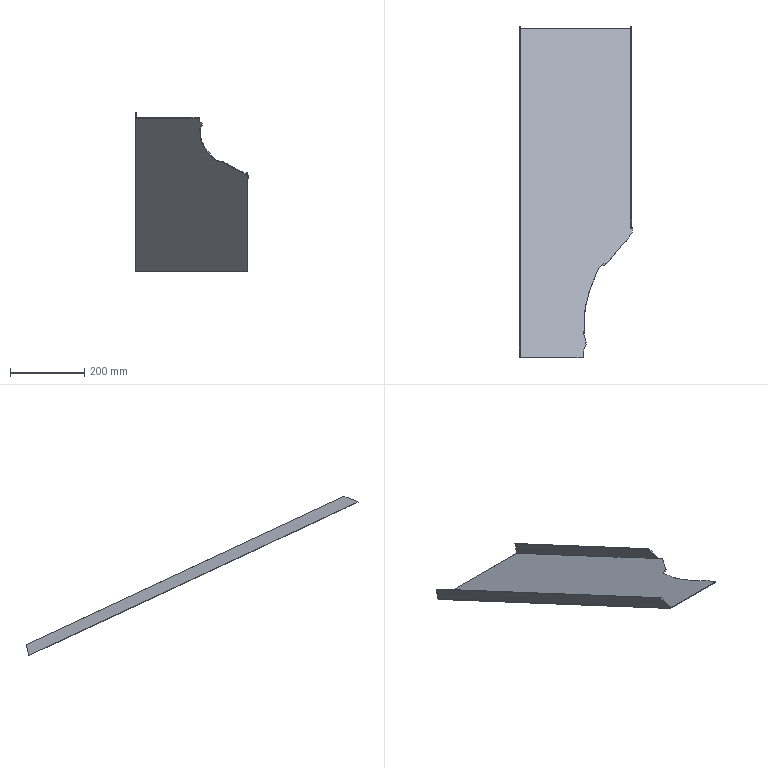Part | NX | features solid 2 | 1 solid | 19 faces | box 305.71 x 896.283 x 429.623 mm | volume 608820 mm3 | spline 10 | plane 9
STEP:
#1=CARTESIAN_POINT('',(-957.116,812.386,-453.753));
#2=VERTEX_POINT('',#1);
#3=CARTESIAN_POINT('',(-957.116,804.502,-483.178));
#4=VERTEX_POINT('',#3);
#5=CARTESIAN_POINT('',(-957.116,798.788,-504.501));
#6=DIRECTION('',(0.,-0.2588,-0.9659));
#7=VECTOR('',#6,1000.);
#8=LINE('',#5,#7);
#9=EDGE_CURVE('',#2,#4,#8,.T.);
#10=ORIENTED_EDGE('',*,*,#9,.F.);
#11=CARTESIAN_POINT('',(-957.116,303.055,-216.248));
#12=VERTEX_POINT('',#11);
#13=CARTESIAN_POINT('',(-957.116,812.386,-453.753));
#14=CARTESIAN_POINT('',(-957.116,642.609,-374.584));
#15=CARTESIAN_POINT('',(-957.116,472.832,-295.416));
#16=CARTESIAN_POINT('',(-957.116,303.055,-216.248));
#17=B_SPLINE_CURVE_WITH_KNOTS('',3,(#13,#14,#15,#16),.UNSPECIFIED.,.F.,.F.,(4,4),(2.402,2.964),.UNSPECIFIED.);
#18=EDGE_CURVE('',#2,#12,#17,.T.);
#19=ORIENTED_EDGE('',*,*,#18,.T.);
#20=CARTESIAN_POINT('',(-957.116,265.845,-229.791));
#21=VERTEX_POINT('',#20);
#22=CARTESIAN_POINT('',(-957.116,753.393,-52.339));
#23=DIRECTION('',(0.,0.9397,0.342));
#24=VECTOR('',#23,1000.);
#25=LINE('',#22,#24);
#26=EDGE_CURVE('',#12,#21,#25,.F.);
#27=ORIENTED_EDGE('',*,*,#26,.T.);
#28=CARTESIAN_POINT('',(-957.116,270.248,-231.844));
#29=VERTEX_POINT('',#28);
#30=CARTESIAN_POINT('',(-957.116,265.845,-229.791));
#31=CARTESIAN_POINT('',(-957.116,267.313,-230.476));
#32=CARTESIAN_POINT('',(-957.116,268.78,-231.16));
#33=CARTESIAN_POINT('',(-957.116,270.248,-231.844));
#34=B_SPLINE_CURVE_WITH_KNOTS('',3,(#30,#31,#32,#33),.UNSPECIFIED.,.F.,.F.,(4,4),(1.938,1.943),.UNSPECIFIED.);
#35=EDGE_CURVE('',#21,#29,#34,.T.);
#36=ORIENTED_EDGE('',*,*,#35,.T.);
#37=CARTESIAN_POINT('',(-957.116,270.248,-234.051));
#38=VERTEX_POINT('',#37);
#39=CARTESIAN_POINT('',(-957.116,270.248,-234.051));
#40=DIRECTION('',(0.,0.,1.));
#41=VECTOR('',#40,1000.);
#42=LINE('',#39,#41);
#43=EDGE_CURVE('',#38,#29,#42,.T.);
#44=ORIENTED_EDGE('',*,*,#43,.F.);
#45=CARTESIAN_POINT('',(-957.116,804.502,-483.178));
#46=CARTESIAN_POINT('',(-957.116,626.417,-400.135));
#47=CARTESIAN_POINT('',(-957.116,448.332,-317.093));
#48=CARTESIAN_POINT('',(-957.116,270.248,-234.051));
#49=B_SPLINE_CURVE_WITH_KNOTS('',3,(#45,#46,#47,#48),.UNSPECIFIED.,.F.,.F.,(4,4),(5.22,5.81),.UNSPECIFIED.);
#50=EDGE_CURVE('',#4,#38,#49,.T.);
#51=ORIENTED_EDGE('',*,*,#50,.F.);
#52=EDGE_LOOP('',(#10,#19,#27,#36,#44,#51));
#53=FACE_BOUND('',#52,.T.);
#54=CARTESIAN_POINT('',(-957.116,930.845,-539.886));
#55=DIRECTION('',(1.,0.,0.));
#56=DIRECTION('',(0.,0.,-1.));
#57=AXIS2_PLACEMENT_3D('',#54,#55,#56);
#58=PLANE('',#57);
#59=ADVANCED_FACE('',(#53),#58,.T.);
#60=CARTESIAN_POINT('',(-959.116,265.845,-229.791));
#61=VERTEX_POINT('',#60);
#62=CARTESIAN_POINT('',(-959.116,805.027,-481.216));
#63=VERTEX_POINT('',#62);
#64=CARTESIAN_POINT('',(-959.116,265.845,-229.791));
#65=CARTESIAN_POINT('',(-959.116,445.573,-313.599));
#66=CARTESIAN_POINT('',(-959.116,625.3,-397.408));
#67=CARTESIAN_POINT('',(-959.116,805.027,-481.216));
#68=B_SPLINE_CURVE_WITH_KNOTS('',3,(#64,#65,#66,#67),.UNSPECIFIED.,.F.,.F.,(4,4),(0.5416,1.136),.UNSPECIFIED.);
#69=EDGE_CURVE('',#61,#63,#68,.T.);
#70=ORIENTED_EDGE('',*,*,#69,.T.);
#71=CARTESIAN_POINT('',(-1258.,805.027,-481.216));
#72=VERTEX_POINT('',#71);
#73=CARTESIAN_POINT('',(-1108.558,805.027,-481.216));
#74=DIRECTION('',(-1.,0.,0.));
#75=VECTOR('',#74,1000.);
#76=LINE('',#73,#75);
#77=EDGE_CURVE('',#63,#72,#76,.T.);
#78=ORIENTED_EDGE('',*,*,#77,.T.);
#79=CARTESIAN_POINT('',(-1258.,-83.052,-67.098));
#80=VERTEX_POINT('',#79);
#81=CARTESIAN_POINT('',(-1258.,805.027,-481.216));
#82=CARTESIAN_POINT('',(-1258.,509.001,-343.176));
#83=CARTESIAN_POINT('',(-1258.,212.974,-205.137));
#84=CARTESIAN_POINT('',(-1258.,-83.052,-67.098));
#85=B_SPLINE_CURVE_WITH_KNOTS('',3,(#81,#82,#83,#84),.UNSPECIFIED.,.F.,.F.,(4,4),(1.577,2.557),.UNSPECIFIED.);
#86=EDGE_CURVE('',#72,#80,#85,.T.);
#87=ORIENTED_EDGE('',*,*,#86,.T.);
#88=CARTESIAN_POINT('',(-1088.022,-83.052,-67.098));
#89=VERTEX_POINT('',#88);
#90=CARTESIAN_POINT('',(-947.116,-83.052,-67.098));
#91=CARTESIAN_POINT('',(-1270.,-83.052,-67.098));
#92=B_SPLINE_CURVE_WITH_KNOTS('',1,(#90,#91),.UNSPECIFIED.,.F.,.F.,(2,2),(0.,1.),.PIECEWISE_BEZIER_KNOTS.);
#93=EDGE_CURVE('',#89,#80,#92,.T.);
#94=ORIENTED_EDGE('',*,*,#93,.F.);
#95=CARTESIAN_POINT('',(-1071.283,94.854,-150.057));
#96=VERTEX_POINT('',#95);
#97=CARTESIAN_POINT('',(-1071.283,94.854,-150.057));
#98=CARTESIAN_POINT('',(-1073.821,87.518,-146.636));
#99=CARTESIAN_POINT('',(-1078.157,72.757,-139.753));
#100=CARTESIAN_POINT('',(-1081.784,54.094,-131.05));
#101=CARTESIAN_POINT('',(-1083.565,39.031,-124.026));
#102=CARTESIAN_POINT('',(-1084.365,27.671,-118.729));
#103=CARTESIAN_POINT('',(-1084.786,16.265,-113.41));
#104=CARTESIAN_POINT('',(-1085.061,6.752,-108.974));
#105=CARTESIAN_POINT('',(-1085.31,-0.8546,-105.427));
#106=CARTESIAN_POINT('',(-1085.507,-6.561,-102.766));
#107=CARTESIAN_POINT('',(-1085.664,-12.263,-100.107));
#108=CARTESIAN_POINT('',(-1086.004,-17.976,-97.443));
#109=CARTESIAN_POINT('',(-1085.683,-22.705,-95.238));
#110=CARTESIAN_POINT('',(-1084.452,-26.233,-93.593));
#111=CARTESIAN_POINT('',(-1083.214,-28.806,-92.393));
#112=CARTESIAN_POINT('',(-1082.034,-31.393,-91.187));
#113=CARTESIAN_POINT('',(-1080.843,-34.932,-89.537));
#114=CARTESIAN_POINT('',(-1079.961,-39.413,-87.447));
#115=CARTESIAN_POINT('',(-1079.819,-44.973,-84.854));
#116=CARTESIAN_POINT('',(-1080.658,-50.409,-82.319));
#117=CARTESIAN_POINT('',(-1082.095,-54.811,-80.267));
#118=CARTESIAN_POINT('',(-1083.811,-58.207,-78.683));
#119=CARTESIAN_POINT('',(-1085.274,-60.705,-77.518));
#120=CARTESIAN_POINT('',(-1086.471,-63.274,-76.321));
#121=CARTESIAN_POINT('',(-1087.46,-66.858,-74.649));
#122=CARTESIAN_POINT('',(-1087.701,-71.602,-72.437));
#123=CARTESIAN_POINT('',(-1087.818,-77.333,-69.765));
#124=CARTESIAN_POINT('',(-1087.961,-81.145,-67.987));
#125=CARTESIAN_POINT('',(-1088.022,-83.052,-67.098));
#126=B_SPLINE_CURVE_WITH_KNOTS('',3,(#97,#98,#99,#100,#101,#102,#103,#104,#105,#106,#107,#108,#109,#110,#111,#112,#113,#114,#115,#116,#117,#118,#119,#120,#121,#122,#123,#124,#125),.UNSPECIFIED.,.F.,.F.,(4,1,1,1,1,1,1,1,1,1,1,1,1,1,1,1,1,1,1,1,1,1,1,1,1,1,4),(0.4038,0.4294,0.4549,0.4677,0.4804,0.4932,0.506,0.5124,0.5187,0.5251,0.5315,0.5379,0.5411,0.5443,0.5475,0.5507,0.5571,0.5634,0.5698,0.5762,0.5794,0.5826,0.5858,0.589,0.5954,0.6017,0.6081),.UNSPECIFIED.);
#127=EDGE_CURVE('',#89,#96,#126,.F.);
#128=ORIENTED_EDGE('',*,*,#127,.T.);
#129=CARTESIAN_POINT('',(-1031.707,169.79,-185.));
#130=VERTEX_POINT('',#129);
#131=CARTESIAN_POINT('',(-1031.707,169.79,-185.));
#132=CARTESIAN_POINT('',(-1033.093,168.618,-184.453));
#133=CARTESIAN_POINT('',(-1035.987,166.389,-183.414));
#134=CARTESIAN_POINT('',(-1040.481,163.191,-181.923));
#135=CARTESIAN_POINT('',(-1044.067,160.372,-180.608));
#136=CARTESIAN_POINT('',(-1046.427,157.646,-179.337));
#137=CARTESIAN_POINT('',(-1048.368,154.491,-177.866));
#138=CARTESIAN_POINT('',(-1049.969,150.289,-175.907));
#139=CARTESIAN_POINT('',(-1051.867,145.236,-173.55));
#140=CARTESIAN_POINT('',(-1053.83,140.205,-171.204));
#141=CARTESIAN_POINT('',(-1056.512,133.517,-168.086));
#142=CARTESIAN_POINT('',(-1059.88,125.163,-164.19));
#143=CARTESIAN_POINT('',(-1063.81,115.101,-159.498));
#144=CARTESIAN_POINT('',(-1067.555,104.981,-154.779));
#145=CARTESIAN_POINT('',(-1070.039,98.229,-151.631));
#146=CARTESIAN_POINT('',(-1071.283,94.854,-150.057));
#147=B_SPLINE_CURVE_WITH_KNOTS('',3,(#131,#132,#133,#134,#135,#136,#137,#138,#139,#140,#141,#142,#143,#144,#145,#146),.UNSPECIFIED.,.F.,.F.,(4,1,1,1,1,1,1,1,1,1,1,1,1,4),(0.,0.005686,0.01137,0.01706,0.0199,0.02274,0.02843,0.03412,0.0398,0.04549,0.05686,0.06823,0.0796,0.09098),.UNSPECIFIED.);
#148=EDGE_CURVE('',#130,#96,#147,.T.);
#149=ORIENTED_EDGE('',*,*,#148,.F.);
#150=CARTESIAN_POINT('',(-1024.566,169.79,-185.));
#151=VERTEX_POINT('',#150);
#152=CARTESIAN_POINT('',(-1024.566,169.79,-185.));
#153=CARTESIAN_POINT('',(-1026.946,169.79,-185.));
#154=CARTESIAN_POINT('',(-1029.326,169.79,-185.));
#155=CARTESIAN_POINT('',(-1031.707,169.79,-185.));
#156=B_SPLINE_CURVE_WITH_KNOTS('',3,(#152,#153,#154,#155),.UNSPECIFIED.,.F.,.F.,(4,4),(0.,0.007141),.UNSPECIFIED.);
#157=EDGE_CURVE('',#151,#130,#156,.T.);
#158=ORIENTED_EDGE('',*,*,#157,.F.);
#159=CARTESIAN_POINT('',(-975.747,228.042,-212.163));
#160=VERTEX_POINT('',#159);
#161=CARTESIAN_POINT('',(-1024.566,169.79,-185.));
#162=CARTESIAN_POINT('',(-1020.096,174.38,-187.141));
#163=CARTESIAN_POINT('',(-1013.264,184.943,-192.066));
#164=CARTESIAN_POINT('',(-1001.045,199.5,-198.854));
#165=CARTESIAN_POINT('',(-988.062,213.534,-205.398));
#166=CARTESIAN_POINT('',(-979.723,223.113,-209.865));
#167=CARTESIAN_POINT('',(-975.747,228.042,-212.163));
#168=B_SPLINE_CURVE_WITH_KNOTS('',3,(#161,#162,#163,#164,#165,#166,#167),.UNSPECIFIED.,.F.,.F.,(4,1,1,1,4),(0.,0.02017,0.04034,0.06051,0.08069),.UNSPECIFIED.);
#169=EDGE_CURVE('',#151,#160,#168,.T.);
#170=ORIENTED_EDGE('',*,*,#169,.T.);
#171=CARTESIAN_POINT('',(-957.225,251.559,-223.129));
#172=VERTEX_POINT('',#171);
#173=CARTESIAN_POINT('',(-975.747,228.042,-212.163));
#174=CARTESIAN_POINT('',(-974.622,228.716,-212.478));
#175=CARTESIAN_POINT('',(-972.462,230.142,-213.143));
#176=CARTESIAN_POINT('',(-969.952,233.079,-214.512));
#177=CARTESIAN_POINT('',(-968.264,236.396,-216.059));
#178=CARTESIAN_POINT('',(-966.441,239.664,-217.582));
#179=CARTESIAN_POINT('',(-964.204,242.681,-218.989));
#180=CARTESIAN_POINT('',(-961.075,246.609,-220.821));
#181=CARTESIAN_POINT('',(-958.769,249.581,-222.207));
#182=CARTESIAN_POINT('',(-957.225,251.559,-223.129));
#183=B_SPLINE_CURVE_WITH_KNOTS('',3,(#173,#174,#175,#176,#177,#178,#179,#180,#181,#182),.UNSPECIFIED.,.F.,.F.,(4,1,1,1,1,1,1,4),(0.,0.004,0.007999,0.012,0.016,0.02,0.024,0.032),.UNSPECIFIED.);
#184=EDGE_CURVE('',#160,#172,#183,.T.);
#185=ORIENTED_EDGE('',*,*,#184,.T.);
#186=CARTESIAN_POINT('',(-955.276,255.196,-224.825));
#187=VERTEX_POINT('',#186);
#188=CARTESIAN_POINT('',(-957.225,251.559,-223.129));
#189=CARTESIAN_POINT('',(-956.4,252.694,-223.659));
#190=CARTESIAN_POINT('',(-955.735,253.899,-224.221));
#191=CARTESIAN_POINT('',(-955.276,255.196,-224.825));
#192=B_SPLINE_CURVE_WITH_KNOTS('',3,(#188,#189,#190,#191),.UNSPECIFIED.,.F.,.F.,(4,4),(0.,0.004461),.UNSPECIFIED.);
#193=EDGE_CURVE('',#172,#187,#192,.T.);
#194=ORIENTED_EDGE('',*,*,#193,.T.);
#195=CARTESIAN_POINT('',(-955.276,255.196,-224.825));
#196=CARTESIAN_POINT('',(-954.837,256.435,-225.403));
#197=CARTESIAN_POINT('',(-954.274,258.981,-226.59));
#198=CARTESIAN_POINT('',(-954.242,262.912,-228.423));
#199=CARTESIAN_POINT('',(-955.033,266.805,-230.239));
#200=CARTESIAN_POINT('',(-956.449,269.093,-231.306));
#201=CARTESIAN_POINT('',(-957.116,270.248,-231.844));
#202=B_SPLINE_CURVE_WITH_KNOTS('',3,(#195,#196,#197,#198,#199,#200,#201),.UNSPECIFIED.,.F.,.F.,(4,1,1,1,4),(0.04957,0.05375,0.05792,0.0621,0.06627),.UNSPECIFIED.);
#203=EDGE_CURVE('',#187,#29,#202,.T.);
#204=ORIENTED_EDGE('',*,*,#203,.T.);
#205=ORIENTED_EDGE('',*,*,#35,.F.);
#206=CARTESIAN_POINT('',(-947.116,265.845,-229.791));
#207=DIRECTION('',(1.,0.,0.));
#208=VECTOR('',#207,1000.);
#209=LINE('',#206,#208);
#210=EDGE_CURVE('',#21,#61,#209,.F.);
#211=ORIENTED_EDGE('',*,*,#210,.T.);
#212=EDGE_LOOP('',(#70,#78,#87,#94,#128,#149,#158,#170,#185,#194,#204,#205,#211));
#213=FACE_BOUND('',#212,.T.);
#214=CARTESIAN_POINT('',(-952.396,-83.052,-67.098));
#215=CARTESIAN_POINT('',(-952.396,805.027,-481.216));
#216=CARTESIAN_POINT('',(-1258.,-83.052,-67.098));
#217=CARTESIAN_POINT('',(-1258.,805.027,-481.216));
#218=B_SPLINE_SURFACE_WITH_KNOTS('',1,1,((#214,#215),(#216,#217)),.PLANE_SURF.,.F.,.F.,.F.,(2,2),(2,2),(0.01635,0.9628),(0.,0.8759),.PIECEWISE_BEZIER_KNOTS.);
#219=ADVANCED_FACE('',(#213),#218,.F.);
#220=CARTESIAN_POINT('',(-1260.,804.502,-483.178));
#221=VERTEX_POINT('',#220);
#222=CARTESIAN_POINT('',(-1108.558,804.502,-483.178));
#223=DIRECTION('',(-1.,0.,0.));
#224=VECTOR('',#223,1000.);
#225=LINE('',#222,#224);
#226=EDGE_CURVE('',#4,#221,#225,.T.);
#227=ORIENTED_EDGE('',*,*,#226,.F.);
#228=ORIENTED_EDGE('',*,*,#50,.T.);
#229=CARTESIAN_POINT('',(-955.276,255.196,-227.032));
#230=VERTEX_POINT('',#229);
#231=CARTESIAN_POINT('',(-955.276,255.196,-227.032));
#232=CARTESIAN_POINT('',(-954.835,256.442,-227.613));
#233=CARTESIAN_POINT('',(-954.271,259.022,-228.816));
#234=CARTESIAN_POINT('',(-954.243,262.874,-230.613));
#235=CARTESIAN_POINT('',(-955.018,266.775,-232.432));
#236=CARTESIAN_POINT('',(-956.443,269.082,-233.507));
#237=CARTESIAN_POINT('',(-957.116,270.248,-234.051));
#238=B_SPLINE_CURVE_WITH_KNOTS('',3,(#231,#232,#233,#234,#235,#236,#237),.UNSPECIFIED.,.F.,.F.,(4,1,1,1,4),(0.02531,0.02954,0.03376,0.03798,0.0422),.UNSPECIFIED.);
#239=EDGE_CURVE('',#230,#38,#238,.T.);
#240=ORIENTED_EDGE('',*,*,#239,.F.);
#241=CARTESIAN_POINT('',(-957.225,251.559,-225.336));
#242=VERTEX_POINT('',#241);
#243=CARTESIAN_POINT('',(-957.225,251.559,-225.336));
#244=CARTESIAN_POINT('',(-956.4,252.694,-225.866));
#245=CARTESIAN_POINT('',(-955.735,253.899,-226.428));
#246=CARTESIAN_POINT('',(-955.276,255.196,-227.032));
#247=B_SPLINE_CURVE_WITH_KNOTS('',3,(#243,#244,#245,#246),.UNSPECIFIED.,.F.,.F.,(4,4),(0.,0.004461),.UNSPECIFIED.);
#248=EDGE_CURVE('',#242,#230,#247,.T.);
#249=ORIENTED_EDGE('',*,*,#248,.F.);
#250=CARTESIAN_POINT('',(-975.747,228.042,-214.37));
#251=VERTEX_POINT('',#250);
#252=CARTESIAN_POINT('',(-975.747,228.042,-214.37));
#253=CARTESIAN_POINT('',(-974.63,228.712,-214.682));
#254=CARTESIAN_POINT('',(-972.438,230.16,-215.358));
#255=CARTESIAN_POINT('',(-969.945,233.094,-216.726));
#256=CARTESIAN_POINT('',(-968.259,236.405,-218.27));
#257=CARTESIAN_POINT('',(-966.436,239.671,-219.793));
#258=CARTESIAN_POINT('',(-964.202,242.683,-221.197));
#259=CARTESIAN_POINT('',(-961.073,246.611,-223.029));
#260=CARTESIAN_POINT('',(-958.768,249.582,-224.414));
#261=CARTESIAN_POINT('',(-957.225,251.559,-225.336));
#262=B_SPLINE_CURVE_WITH_KNOTS('',3,(#252,#253,#254,#255,#256,#257,#258,#259,#260,#261),.UNSPECIFIED.,.F.,.F.,(4,1,1,1,1,1,1,4),(0.1165,0.1206,0.1246,0.1286,0.1326,0.1366,0.1406,0.1487),.UNSPECIFIED.);
#263=EDGE_CURVE('',#251,#242,#262,.T.);
#264=ORIENTED_EDGE('',*,*,#263,.F.);
#265=CARTESIAN_POINT('',(-1029.771,165.058,-185.));
#266=VERTEX_POINT('',#265);
#267=CARTESIAN_POINT('',(-1029.771,165.058,-185.));
#268=CARTESIAN_POINT('',(-1026.992,167.315,-186.053));
#269=CARTESIAN_POINT('',(-1021.935,172.205,-188.333));
#270=CARTESIAN_POINT('',(-1015.967,180.594,-192.245));
#271=CARTESIAN_POINT('',(-1009.886,188.91,-196.122));
#272=CARTESIAN_POINT('',(-1003.235,196.853,-199.826));
#273=CARTESIAN_POINT('',(-996.292,204.603,-203.44));
#274=CARTESIAN_POINT('',(-986.933,214.866,-208.226));
#275=CARTESIAN_POINT('',(-980.077,222.674,-211.867));
#276=CARTESIAN_POINT('',(-975.747,228.042,-214.37));
#277=B_SPLINE_CURVE_WITH_KNOTS('',3,(#267,#268,#269,#270,#271,#272,#273,#274,#275,#276),.UNSPECIFIED.,.F.,.F.,(4,1,1,1,1,1,1,4),(0.1682,0.1798,0.1914,0.2031,0.2147,0.2263,0.2379,0.2611),.UNSPECIFIED.);
#278=EDGE_CURVE('',#266,#251,#277,.T.);
#279=ORIENTED_EDGE('',*,*,#278,.F.);
#280=CARTESIAN_POINT('',(-1037.859,165.058,-185.));
#281=VERTEX_POINT('',#280);
#282=CARTESIAN_POINT('',(-1029.771,165.058,-185.));
#283=CARTESIAN_POINT('',(-1032.467,165.058,-185.));
#284=CARTESIAN_POINT('',(-1035.163,165.058,-185.));
#285=CARTESIAN_POINT('',(-1037.859,165.058,-185.));
#286=B_SPLINE_CURVE_WITH_KNOTS('',3,(#282,#283,#284,#285),.UNSPECIFIED.,.F.,.F.,(4,4),(0.,0.008088),.UNSPECIFIED.);
#287=EDGE_CURVE('',#266,#281,#286,.T.);
#288=ORIENTED_EDGE('',*,*,#287,.T.);
#289=CARTESIAN_POINT('',(-1071.283,94.854,-152.264));
#290=VERTEX_POINT('',#289);
#291=CARTESIAN_POINT('',(-1071.283,94.854,-152.264));
#292=CARTESIAN_POINT('',(-1070.155,97.916,-153.691));
#293=CARTESIAN_POINT('',(-1067.898,104.041,-156.547));
#294=CARTESIAN_POINT('',(-1064.514,113.227,-160.831));
#295=CARTESIAN_POINT('',(-1060.983,122.369,-165.094));
#296=CARTESIAN_POINT('',(-1057.342,131.477,-169.341));
#297=CARTESIAN_POINT('',(-1053.661,140.571,-173.582));
#298=CARTESIAN_POINT('',(-1050.739,148.199,-177.138));
#299=CARTESIAN_POINT('',(-1048.466,154.317,-179.992));
#300=CARTESIAN_POINT('',(-1045.937,158.571,-181.975));
#301=CARTESIAN_POINT('',(-1042.052,162.047,-183.596));
#302=CARTESIAN_POINT('',(-1039.253,164.042,-184.526));
#303=CARTESIAN_POINT('',(-1037.859,165.058,-185.));
#304=B_SPLINE_CURVE_WITH_KNOTS('',3,(#291,#292,#293,#294,#295,#296,#297,#298,#299,#300,#301,#302,#303),.UNSPECIFIED.,.F.,.F.,(4,1,1,1,1,1,1,1,1,1,4),(0.4296,0.4403,0.451,0.4617,0.4723,0.483,0.4937,0.4991,0.5044,0.5098,0.5151),.UNSPECIFIED.);
#305=EDGE_CURVE('',#281,#290,#304,.F.);
#306=ORIENTED_EDGE('',*,*,#305,.T.);
#307=CARTESIAN_POINT('',(-1088.049,-83.898,-68.91));
#308=VERTEX_POINT('',#307);
#309=CARTESIAN_POINT('',(-1088.049,-83.898,-68.91));
#310=CARTESIAN_POINT('',(-1087.992,-82.107,-69.745));
#311=CARTESIAN_POINT('',(-1087.876,-78.527,-71.414));
#312=CARTESIAN_POINT('',(-1087.693,-73.156,-73.919));
#313=CARTESIAN_POINT('',(-1087.611,-67.782,-76.425));
#314=CARTESIAN_POINT('',(-1086.426,-62.488,-78.894));
#315=CARTESIAN_POINT('',(-1083.252,-57.464,-81.236));
#316=CARTESIAN_POINT('',(-1081.123,-52.203,-83.689));
#317=CARTESIAN_POINT('',(-1079.949,-46.553,-86.324));
#318=CARTESIAN_POINT('',(-1079.826,-40.873,-88.973));
#319=CARTESIAN_POINT('',(-1080.675,-35.228,-91.605));
#320=CARTESIAN_POINT('',(-1082.321,-30.578,-93.774));
#321=CARTESIAN_POINT('',(-1084.162,-26.901,-95.488));
#322=CARTESIAN_POINT('',(-1085.594,-23.193,-97.217));
#323=CARTESIAN_POINT('',(-1086.022,-18.455,-99.427));
#324=CARTESIAN_POINT('',(-1085.685,-12.704,-102.108));
#325=CARTESIAN_POINT('',(-1085.519,-6.967,-104.783));
#326=CARTESIAN_POINT('',(-1085.324,-1.228,-107.46));
#327=CARTESIAN_POINT('',(-1085.071,6.424,-111.028));
#328=CARTESIAN_POINT('',(-1084.794,15.988,-115.488));
#329=CARTESIAN_POINT('',(-1084.377,27.456,-120.835));
#330=CARTESIAN_POINT('',(-1083.581,38.873,-126.159));
#331=CARTESIAN_POINT('',(-1081.801,54.,-133.213));
#332=CARTESIAN_POINT('',(-1078.167,72.722,-141.943));
#333=CARTESIAN_POINT('',(-1073.824,87.511,-148.839));
#334=CARTESIAN_POINT('',(-1071.283,94.854,-152.264));
#335=B_SPLINE_CURVE_WITH_KNOTS('',3,(#309,#310,#311,#312,#313,#314,#315,#316,#317,#318,#319,#320,#321,#322,#323,#324,#325,#326,#327,#328,#329,#330,#331,#332,#333,#334),.UNSPECIFIED.,.F.,.F.,(4,1,1,1,1,1,1,1,1,1,1,1,1,1,1,1,1,1,1,1,1,1,1,4),(0.,0.005912,0.01182,0.01774,0.02365,0.02956,0.03547,0.04139,0.0473,0.05321,0.05912,0.06208,0.06504,0.07095,0.07686,0.08277,0.08868,0.0946,0.1064,0.1182,0.1301,0.1419,0.1655,0.1892),.UNSPECIFIED.);
#336=EDGE_CURVE('',#308,#290,#335,.T.);
#337=ORIENTED_EDGE('',*,*,#336,.F.);
#338=CARTESIAN_POINT('',(-1260.,-83.898,-68.91));
#339=VERTEX_POINT('',#338);
#340=CARTESIAN_POINT('',(-947.116,-83.898,-68.91));
#341=CARTESIAN_POINT('',(-1270.,-83.898,-68.91));
#342=B_SPLINE_CURVE_WITH_KNOTS('',1,(#340,#341),.UNSPECIFIED.,.F.,.F.,(2,2),(0.,1.),.PIECEWISE_BEZIER_KNOTS.);
#343=EDGE_CURVE('',#308,#339,#342,.T.);
#344=ORIENTED_EDGE('',*,*,#343,.T.);
#345=CARTESIAN_POINT('',(-1260.,-83.898,-68.91));
#346=CARTESIAN_POINT('',(-1260.,212.235,-206.999));
#347=CARTESIAN_POINT('',(-1260.,508.369,-345.088));
#348=CARTESIAN_POINT('',(-1260.,804.502,-483.178));
#349=B_SPLINE_CURVE_WITH_KNOTS('',3,(#345,#346,#347,#348),.UNSPECIFIED.,.F.,.F.,(4,4),(4.96,5.941),.UNSPECIFIED.);
#350=EDGE_CURVE('',#339,#221,#349,.T.);
#351=ORIENTED_EDGE('',*,*,#350,.T.);
#352=EDGE_LOOP('',(#227,#228,#240,#249,#264,#279,#288,#306,#337,#344,#351));
#353=FACE_BOUND('',#352,.T.);
#354=CARTESIAN_POINT('',(-952.294,-83.898,-68.91));
#355=CARTESIAN_POINT('',(-952.294,804.502,-483.178));
#356=CARTESIAN_POINT('',(-1260.,-83.898,-68.91));
#357=CARTESIAN_POINT('',(-1260.,804.502,-483.178));
#358=B_SPLINE_SURFACE_WITH_KNOTS('',1,1,((#354,#355),(#356,#357)),.PLANE_SURF.,.F.,.F.,.F.,(2,2),(2,2),(0.01604,0.969),(0.,0.8762),.PIECEWISE_BEZIER_KNOTS.);
#359=ADVANCED_FACE('',(#353),#358,.T.);
#360=ORIENTED_EDGE('',*,*,#93,.T.);
#361=CARTESIAN_POINT('',(-1260.,-83.052,-67.098));
#362=VERTEX_POINT('',#361);
#363=CARTESIAN_POINT('',(-1270.,-83.052,-67.098));
#364=DIRECTION('',(1.,0.,0.));
#365=VECTOR('',#364,1000.);
#366=LINE('',#363,#365);
#367=EDGE_CURVE('',#80,#362,#366,.F.);
#368=ORIENTED_EDGE('',*,*,#367,.T.);
#369=CARTESIAN_POINT('',(-1260.,-83.052,-67.098));
#370=DIRECTION('',(0.,-0.4226,-0.9063));
#371=VECTOR('',#370,1000.);
#372=LINE('',#369,#371);
#373=EDGE_CURVE('',#362,#339,#372,.T.);
#374=ORIENTED_EDGE('',*,*,#373,.T.);
#375=ORIENTED_EDGE('',*,*,#343,.F.);
#376=CARTESIAN_POINT('',(-1088.022,-83.052,-67.098));
#377=CARTESIAN_POINT('',(-1088.031,-83.334,-67.702));
#378=CARTESIAN_POINT('',(-1088.04,-83.616,-68.306));
#379=CARTESIAN_POINT('',(-1088.049,-83.898,-68.91));
#380=B_SPLINE_CURVE_WITH_KNOTS('',3,(#376,#377,#378,#379),.UNSPECIFIED.,.F.,.F.,(4,4),(0.00999,0.01199),.UNSPECIFIED.);
#381=EDGE_CURVE('',#89,#308,#380,.T.);
#382=ORIENTED_EDGE('',*,*,#381,.F.);
#383=EDGE_LOOP('',(#360,#368,#374,#375,#382));
#384=FACE_BOUND('',#383,.T.);
#385=CARTESIAN_POINT('',(-947.116,-83.052,-67.098));
#386=DIRECTION('',(0.,-0.9063,0.4226));
#387=DIRECTION('',(0.,-0.4226,-0.9063));
#388=AXIS2_PLACEMENT_3D('',#385,#386,#387);
#389=PLANE('',#388);
#390=ADVANCED_FACE('',(#384),#389,.T.);
#391=CARTESIAN_POINT('',(-1260.,812.386,-453.753));
#392=VERTEX_POINT('',#391);
#393=CARTESIAN_POINT('',(-1260.,849.067,-316.858));
#394=DIRECTION('',(0.,0.2588,0.9659));
#395=VECTOR('',#394,1000.);
#396=LINE('',#393,#395);
#397=EDGE_CURVE('',#221,#392,#396,.T.);
#398=ORIENTED_EDGE('',*,*,#397,.F.);
#399=ORIENTED_EDGE('',*,*,#350,.F.);
#400=ORIENTED_EDGE('',*,*,#373,.F.);
#401=CARTESIAN_POINT('',(-1260.,-45.842,-53.554));
#402=VERTEX_POINT('',#401);
#403=CARTESIAN_POINT('',(-1260.,-83.052,-67.098));
#404=DIRECTION('',(0.,-0.9397,-0.342));
#405=VECTOR('',#404,1000.);
#406=LINE('',#403,#405);
#407=EDGE_CURVE('',#362,#402,#406,.F.);
#408=ORIENTED_EDGE('',*,*,#407,.T.);
#409=CARTESIAN_POINT('',(-1260.,-45.842,-53.554));
#410=CARTESIAN_POINT('',(-1260.,240.234,-186.954));
#411=CARTESIAN_POINT('',(-1260.,526.31,-320.353));
#412=CARTESIAN_POINT('',(-1260.,812.386,-453.753));
#413=B_SPLINE_CURVE_WITH_KNOTS('',3,(#409,#410,#411,#412),.UNSPECIFIED.,.F.,.F.,(4,4),(4.988,5.935),.UNSPECIFIED.);
#414=EDGE_CURVE('',#402,#392,#413,.T.);
#415=ORIENTED_EDGE('',*,*,#414,.T.);
#416=EDGE_LOOP('',(#398,#399,#400,#408,#415));
#417=FACE_BOUND('',#416,.T.);
#418=CARTESIAN_POINT('',(-1260.,-83.052,-67.098));
#419=DIRECTION('',(-1.,0.,0.));
#420=DIRECTION('',(0.,0.,1.));
#421=AXIS2_PLACEMENT_3D('',#418,#419,#420);
#422=PLANE('',#421);
#423=ADVANCED_FACE('',(#417),#422,.T.);
#424=ORIENTED_EDGE('',*,*,#287,.F.);
#425=CARTESIAN_POINT('',(-1024.566,169.79,-185.));
#426=CARTESIAN_POINT('',(-1026.193,168.119,-185.));
#427=CARTESIAN_POINT('',(-1027.936,166.548,-185.));
#428=CARTESIAN_POINT('',(-1029.771,165.058,-185.));
#429=B_SPLINE_CURVE_WITH_KNOTS('',3,(#425,#426,#427,#428),.UNSPECIFIED.,.F.,.F.,(4,4),(0.08025,0.08723),.UNSPECIFIED.);
#430=EDGE_CURVE('',#266,#151,#429,.F.);
#431=ORIENTED_EDGE('',*,*,#430,.T.);
#432=ORIENTED_EDGE('',*,*,#157,.T.);
#433=CARTESIAN_POINT('',(-1037.859,165.058,-185.));
#434=CARTESIAN_POINT('',(-1035.768,166.582,-185.));
#435=CARTESIAN_POINT('',(-1033.684,168.117,-185.));
#436=CARTESIAN_POINT('',(-1031.707,169.79,-185.));
#437=B_SPLINE_CURVE_WITH_KNOTS('',3,(#433,#434,#435,#436),.UNSPECIFIED.,.F.,.F.,(4,4),(0.,0.007762),.UNSPECIFIED.);
#438=EDGE_CURVE('',#281,#130,#437,.T.);
#439=ORIENTED_EDGE('',*,*,#438,.F.);
#440=EDGE_LOOP('',(#424,#431,#432,#439));
#441=FACE_BOUND('',#440,.T.);
#442=CARTESIAN_POINT('',(-1097.567,-373.462,-185.));
#443=DIRECTION('',(0.,0.,1.));
#444=DIRECTION('',(1.,0.,0.));
#445=AXIS2_PLACEMENT_3D('',#442,#443,#444);
#446=PLANE('',#445);
#447=ADVANCED_FACE('',(#441),#446,.T.);
#448=ORIENTED_EDGE('',*,*,#148,.T.);
#449=CARTESIAN_POINT('',(-1071.283,94.854,-152.264));
#450=DIRECTION('',(0.,0.,-1.));
#451=VECTOR('',#450,1000.);
#452=LINE('',#449,#451);
#453=EDGE_CURVE('',#290,#96,#452,.F.);
#454=ORIENTED_EDGE('',*,*,#453,.F.);
#455=ORIENTED_EDGE('',*,*,#305,.F.);
#456=ORIENTED_EDGE('',*,*,#438,.T.);
#457=EDGE_LOOP('',(#448,#454,#455,#456));
#458=FACE_BOUND('',#457,.T.);
#459=CARTESIAN_POINT('',(-1031.3,170.138,-175.152));
#460=CARTESIAN_POINT('',(-1031.3,170.138,-187.286));
#461=CARTESIAN_POINT('',(-1032.716,168.917,-174.732));
#462=CARTESIAN_POINT('',(-1032.716,168.917,-186.866));
#463=CARTESIAN_POINT('',(-1035.655,166.634,-173.799));
#464=CARTESIAN_POINT('',(-1035.655,166.634,-185.933));
#465=CARTESIAN_POINT('',(-1040.138,163.426,-172.189));
#466=CARTESIAN_POINT('',(-1040.138,163.426,-184.323));
#467=CARTESIAN_POINT('',(-1044.57,160.053,-170.666));
#468=CARTESIAN_POINT('',(-1044.57,160.053,-182.8));
#469=CARTESIAN_POINT('',(-1047.95,155.588,-169.139));
#470=CARTESIAN_POINT('',(-1047.95,155.588,-181.273));
#471=CARTESIAN_POINT('',(-1049.905,150.456,-167.34));
#472=CARTESIAN_POINT('',(-1049.905,150.456,-179.474));
#473=CARTESIAN_POINT('',(-1051.776,145.477,-165.174));
#474=CARTESIAN_POINT('',(-1051.776,145.477,-177.308));
#475=CARTESIAN_POINT('',(-1053.688,140.564,-162.878));
#476=CARTESIAN_POINT('',(-1053.688,140.564,-175.012));
#477=CARTESIAN_POINT('',(-1055.646,135.674,-160.577));
#478=CARTESIAN_POINT('',(-1055.646,135.674,-172.711));
#479=CARTESIAN_POINT('',(-1057.616,130.78,-158.294));
#480=CARTESIAN_POINT('',(-1057.616,130.78,-170.427));
#481=CARTESIAN_POINT('',(-1059.578,125.881,-156.014));
#482=CARTESIAN_POINT('',(-1059.578,125.881,-168.148));
#483=CARTESIAN_POINT('',(-1061.518,120.969,-153.746));
#484=CARTESIAN_POINT('',(-1061.518,120.969,-165.88));
#485=CARTESIAN_POINT('',(-1063.099,116.882,-151.802));
#486=CARTESIAN_POINT('',(-1063.099,116.882,-163.936));
#487=CARTESIAN_POINT('',(-1064.339,113.621,-150.172));
#488=CARTESIAN_POINT('',(-1064.339,113.621,-162.305));
#489=CARTESIAN_POINT('',(-1065.283,111.114,-149.187));
#490=CARTESIAN_POINT('',(-1065.283,111.114,-161.321));
#491=CARTESIAN_POINT('',(-1066.257,108.498,-148.758));
#492=CARTESIAN_POINT('',(-1066.257,108.498,-160.892));
#493=CARTESIAN_POINT('',(-1067.6,104.848,-149.156));
#494=CARTESIAN_POINT('',(-1067.6,104.848,-161.29));
#495=CARTESIAN_POINT('',(-1069.273,100.31,-149.504));
#496=CARTESIAN_POINT('',(-1069.273,100.31,-161.638));
#497=CARTESIAN_POINT('',(-1070.613,96.672,-149.829));
#498=CARTESIAN_POINT('',(-1070.613,96.672,-161.962));
#499=CARTESIAN_POINT('',(-1071.283,94.854,-149.985));
#500=CARTESIAN_POINT('',(-1071.283,94.854,-162.119));
#501=B_SPLINE_SURFACE_WITH_KNOTS('',3,1,((#459,#460),(#461,#462),(#463,#464),(#465,#466),(#467,#468),(#469,#470),(#471,#472),(#473,#474),(#475,#476),(#477,#478),(#479,#480),(#481,#482),(#483,#484),(#485,#486),(#487,#488),(#489,#490),(#491,#492),(#493,#494),(#495,#496),(#497,#498),(#499,#500)),.SURF_OF_LINEAR_EXTRUSION.,.F.,.F.,.F.,(4,1,1,1,1,1,1,1,1,1,1,1,1,1,1,1,1,1,4),(2,2),(0.5749,0.6059,0.6369,0.6679,0.6989,0.7298,0.7608,0.7918,0.8228,0.8538,0.8847,0.9157,0.9467,0.9622,0.9777,0.9932,1.009,1.04,1.071),(0.,1.),.UNSPECIFIED.);
#502=ADVANCED_FACE('',(#458),#501,.T.);
#503=ORIENTED_EDGE('',*,*,#381,.T.);
#504=ORIENTED_EDGE('',*,*,#336,.T.);
#505=ORIENTED_EDGE('',*,*,#453,.T.);
#506=ORIENTED_EDGE('',*,*,#127,.F.);
#507=EDGE_LOOP('',(#503,#504,#505,#506));
#508=FACE_BOUND('',#507,.T.);
#509=CARTESIAN_POINT('',(-1088.084,-84.993,-66.657));
#510=CARTESIAN_POINT('',(-1088.084,-84.993,-169.326));
#511=CARTESIAN_POINT('',(-1088.023,-83.08,-66.491));
#512=CARTESIAN_POINT('',(-1088.023,-83.08,-169.161));
#513=CARTESIAN_POINT('',(-1087.905,-79.251,-66.161));
#514=CARTESIAN_POINT('',(-1087.905,-79.251,-168.83));
#515=CARTESIAN_POINT('',(-1087.688,-73.515,-65.662));
#516=CARTESIAN_POINT('',(-1087.688,-73.515,-168.331));
#517=CARTESIAN_POINT('',(-1087.65,-67.757,-65.178));
#518=CARTESIAN_POINT('',(-1087.65,-67.757,-167.848));
#519=CARTESIAN_POINT('',(-1086.265,-62.116,-64.636));
#520=CARTESIAN_POINT('',(-1086.265,-62.116,-167.306));
#521=CARTESIAN_POINT('',(-1083.124,-57.265,-63.987));
#522=CARTESIAN_POINT('',(-1083.124,-57.265,-166.656));
#523=CARTESIAN_POINT('',(-1081.04,-51.908,-63.33));
#524=CARTESIAN_POINT('',(-1081.04,-51.908,-165.999));
#525=CARTESIAN_POINT('',(-1079.914,-46.261,-62.728));
#526=CARTESIAN_POINT('',(-1079.914,-46.261,-165.397));
#527=CARTESIAN_POINT('',(-1079.848,-40.5,-62.198));
#528=CARTESIAN_POINT('',(-1079.848,-40.5,-164.867));
#529=CARTESIAN_POINT('',(-1080.777,-34.79,-61.786));
#530=CARTESIAN_POINT('',(-1080.777,-34.79,-164.455));
#531=CARTESIAN_POINT('',(-1082.821,-29.405,-61.475));
#532=CARTESIAN_POINT('',(-1082.821,-29.405,-164.144));
#533=CARTESIAN_POINT('',(-1085.498,-24.237,-61.279));
#534=CARTESIAN_POINT('',(-1085.498,-24.237,-163.949));
#535=CARTESIAN_POINT('',(-1086.024,-18.429,-60.902));
#536=CARTESIAN_POINT('',(-1086.024,-18.429,-163.572));
#537=CARTESIAN_POINT('',(-1085.684,-12.703,-60.412));
#538=CARTESIAN_POINT('',(-1085.684,-12.703,-163.081));
#539=CARTESIAN_POINT('',(-1085.519,-6.959,-59.908));
#540=CARTESIAN_POINT('',(-1085.519,-6.959,-162.578));
#541=CARTESIAN_POINT('',(-1085.323,-1.219,-59.414));
#542=CARTESIAN_POINT('',(-1085.323,-1.219,-162.084));
#543=CARTESIAN_POINT('',(-1085.071,6.436,-58.752));
#544=CARTESIAN_POINT('',(-1085.071,6.436,-161.421));
#545=CARTESIAN_POINT('',(-1084.793,16.005,-57.925));
#546=CARTESIAN_POINT('',(-1084.793,16.005,-160.595));
#547=CARTESIAN_POINT('',(-1084.376,27.486,-56.934));
#548=CARTESIAN_POINT('',(-1084.376,27.486,-159.604));
#549=CARTESIAN_POINT('',(-1083.575,38.945,-55.908));
#550=CARTESIAN_POINT('',(-1083.575,38.945,-158.577));
#551=CARTESIAN_POINT('',(-1081.779,54.153,-54.488));
#552=CARTESIAN_POINT('',(-1081.779,54.153,-157.157));
#553=CARTESIAN_POINT('',(-1078.112,72.948,-52.613));
#554=CARTESIAN_POINT('',(-1078.112,72.948,-155.282));
#555=CARTESIAN_POINT('',(-1073.782,87.631,-51.02));
#556=CARTESIAN_POINT('',(-1073.782,87.631,-153.69));
#557=CARTESIAN_POINT('',(-1071.283,94.854,-50.203));
#558=CARTESIAN_POINT('',(-1071.283,94.854,-152.872));
#559=B_SPLINE_SURFACE_WITH_KNOTS('',3,1,((#509,#510),(#511,#512),(#513,#514),(#515,#516),(#517,#518),(#519,#520),(#521,#522),(#523,#524),(#525,#526),(#527,#528),(#529,#530),(#531,#532),(#533,#534),(#535,#536),(#537,#538),(#539,#540),(#541,#542),(#543,#544),(#545,#546),(#547,#548),(#549,#550),(#551,#552),(#553,#554),(#555,#556),(#557,#558)),.SURF_OF_LINEAR_EXTRUSION.,.F.,.F.,.F.,(4,1,1,1,1,1,1,1,1,1,1,1,1,1,1,1,1,1,1,1,1,1,4),(2,2),(0.3734,0.3924,0.4115,0.4305,0.4495,0.4685,0.4875,0.5065,0.5255,0.5446,0.5636,0.5826,0.6016,0.6206,0.6396,0.6586,0.6777,0.7157,0.7537,0.7917,0.8298,0.9058,0.9819),(0.,1.),.UNSPECIFIED.);
#560=ADVANCED_FACE('',(#508),#559,.F.);
#561=CARTESIAN_POINT('',(-975.747,228.042,-214.37));
#562=DIRECTION('',(0.,0.,-1.));
#563=VECTOR('',#562,1000.);
#564=LINE('',#561,#563);
#565=EDGE_CURVE('',#251,#160,#564,.F.);
#566=ORIENTED_EDGE('',*,*,#565,.F.);
#567=ORIENTED_EDGE('',*,*,#263,.T.);
#568=CARTESIAN_POINT('',(-957.225,251.559,-225.336));
#569=DIRECTION('',(0.,0.,-1.));
#570=VECTOR('',#569,1000.);
#571=LINE('',#568,#570);
#572=EDGE_CURVE('',#242,#172,#571,.F.);
#573=ORIENTED_EDGE('',*,*,#572,.T.);
#574=ORIENTED_EDGE('',*,*,#184,.F.);
#575=EDGE_LOOP('',(#566,#567,#573,#574));
#576=FACE_BOUND('',#575,.T.);
#577=CARTESIAN_POINT('',(-957.225,251.559,-225.415));
#578=CARTESIAN_POINT('',(-957.225,251.559,-212.084));
#579=CARTESIAN_POINT('',(-958.07,250.477,-225.415));
#580=CARTESIAN_POINT('',(-958.07,250.477,-212.084));
#581=CARTESIAN_POINT('',(-959.779,248.289,-225.415));
#582=CARTESIAN_POINT('',(-959.779,248.289,-212.084));
#583=CARTESIAN_POINT('',(-961.99,245.462,-225.415));
#584=CARTESIAN_POINT('',(-961.99,245.462,-212.084));
#585=CARTESIAN_POINT('',(-963.943,242.982,-225.415));
#586=CARTESIAN_POINT('',(-963.943,242.982,-212.084));
#587=CARTESIAN_POINT('',(-965.174,241.399,-225.415));
#588=CARTESIAN_POINT('',(-965.174,241.399,-212.084));
#589=CARTESIAN_POINT('',(-965.946,240.3,-225.415));
#590=CARTESIAN_POINT('',(-965.946,240.3,-212.084));
#591=CARTESIAN_POINT('',(-966.586,239.284,-225.415));
#592=CARTESIAN_POINT('',(-966.586,239.284,-212.084));
#593=CARTESIAN_POINT('',(-967.116,238.402,-225.415));
#594=CARTESIAN_POINT('',(-967.116,238.402,-212.084));
#595=CARTESIAN_POINT('',(-967.619,237.524,-225.415));
#596=CARTESIAN_POINT('',(-967.619,237.524,-212.084));
#597=CARTESIAN_POINT('',(-968.039,236.768,-225.415));
#598=CARTESIAN_POINT('',(-968.039,236.768,-212.084));
#599=CARTESIAN_POINT('',(-968.473,235.952,-225.415));
#600=CARTESIAN_POINT('',(-968.473,235.952,-212.084));
#601=CARTESIAN_POINT('',(-968.836,235.264,-225.415));
#602=CARTESIAN_POINT('',(-968.836,235.264,-212.084));
#603=CARTESIAN_POINT('',(-969.191,234.625,-225.415));
#604=CARTESIAN_POINT('',(-969.191,234.625,-212.084));
#605=CARTESIAN_POINT('',(-969.461,234.16,-225.415));
#606=CARTESIAN_POINT('',(-969.461,234.16,-212.084));
#607=CARTESIAN_POINT('',(-969.664,233.819,-225.415));
#608=CARTESIAN_POINT('',(-969.664,233.819,-212.084));
#609=CARTESIAN_POINT('',(-969.809,233.581,-225.415));
#610=CARTESIAN_POINT('',(-969.809,233.581,-212.084));
#611=CARTESIAN_POINT('',(-969.875,233.474,-225.415));
#612=CARTESIAN_POINT('',(-969.875,233.474,-212.084));
#613=CARTESIAN_POINT('',(-970.114,233.097,-225.415));
#614=CARTESIAN_POINT('',(-970.114,233.097,-212.084));
#615=CARTESIAN_POINT('',(-970.446,232.621,-225.415));
#616=CARTESIAN_POINT('',(-970.446,232.621,-212.084));
#617=CARTESIAN_POINT('',(-971.062,231.823,-225.415));
#618=CARTESIAN_POINT('',(-971.062,231.823,-212.084));
#619=CARTESIAN_POINT('',(-971.911,230.882,-225.415));
#620=CARTESIAN_POINT('',(-971.911,230.882,-212.084));
#621=CARTESIAN_POINT('',(-973.034,229.851,-225.415));
#622=CARTESIAN_POINT('',(-973.034,229.851,-212.084));
#623=CARTESIAN_POINT('',(-974.096,229.058,-225.415));
#624=CARTESIAN_POINT('',(-974.096,229.058,-212.084));
#625=CARTESIAN_POINT('',(-974.857,228.57,-225.415));
#626=CARTESIAN_POINT('',(-974.857,228.57,-212.084));
#627=CARTESIAN_POINT('',(-975.461,228.214,-225.415));
#628=CARTESIAN_POINT('',(-975.461,228.214,-212.084));
#629=CARTESIAN_POINT('',(-975.747,228.042,-225.415));
#630=CARTESIAN_POINT('',(-975.747,228.042,-212.084));
#631=B_SPLINE_SURFACE_WITH_KNOTS('',3,1,((#577,#578),(#579,#580),(#581,#582),(#583,#584),(#585,#586),(#587,#588),(#589,#590),(#591,#592),(#593,#594),(#595,#596),(#597,#598),(#599,#600),(#601,#602),(#603,#604),(#605,#606),(#607,#608),(#609,#610),(#611,#612),(#613,#614),(#615,#616),(#617,#618),(#619,#620),(#621,#622),(#623,#624),(#625,#626),(#627,#628),(#629,#630)),.SURF_OF_LINEAR_EXTRUSION.,.F.,.F.,.F.,(4,1,1,1,1,1,1,1,1,1,1,1,1,1,1,1,1,1,1,1,1,1,1,1,4),(2,2),(0.07719,0.0794,0.08162,0.08273,0.08384,0.08494,0.0855,0.08605,0.08661,0.08716,0.08771,0.08827,0.08854,0.08882,0.08896,0.08903,0.0891,0.08938,0.08993,0.09048,0.09159,0.0927,0.09381,0.09436,0.09492),(0.,1.),.UNSPECIFIED.);
#632=ADVANCED_FACE('',(#576),#631,.F.);
#633=CARTESIAN_POINT('',(-955.276,255.196,-224.825));
#634=CARTESIAN_POINT('',(-955.276,255.196,-225.561));
#635=CARTESIAN_POINT('',(-955.276,255.196,-226.296));
#636=CARTESIAN_POINT('',(-955.276,255.196,-227.032));
#637=B_SPLINE_CURVE_WITH_KNOTS('',3,(#633,#634,#635,#636),.UNSPECIFIED.,.F.,.F.,(4,4),(0.3524,1.352),.UNSPECIFIED.);
#638=EDGE_CURVE('',#187,#230,#637,.T.);
#639=ORIENTED_EDGE('',*,*,#638,.T.);
#640=ORIENTED_EDGE('',*,*,#239,.T.);
#641=ORIENTED_EDGE('',*,*,#43,.T.);
#642=ORIENTED_EDGE('',*,*,#203,.F.);
#643=EDGE_LOOP('',(#639,#640,#641,#642));
#644=FACE_BOUND('',#643,.T.);
#645=CARTESIAN_POINT('',(-957.116,270.248,-234.106));
#646=CARTESIAN_POINT('',(-957.116,270.248,-224.77));
#647=CARTESIAN_POINT('',(-956.898,269.87,-234.106));
#648=CARTESIAN_POINT('',(-956.898,269.87,-224.77));
#649=CARTESIAN_POINT('',(-956.573,269.308,-234.106));
#650=CARTESIAN_POINT('',(-956.573,269.308,-224.77));
#651=CARTESIAN_POINT('',(-956.182,268.629,-234.106));
#652=CARTESIAN_POINT('',(-956.182,268.629,-224.77));
#653=CARTESIAN_POINT('',(-955.975,268.273,-234.106));
#654=CARTESIAN_POINT('',(-955.975,268.273,-224.77));
#655=CARTESIAN_POINT('',(-955.866,268.075,-234.106));
#656=CARTESIAN_POINT('',(-955.866,268.075,-224.77));
#657=CARTESIAN_POINT('',(-955.702,267.762,-234.106));
#658=CARTESIAN_POINT('',(-955.702,267.762,-224.77));
#659=CARTESIAN_POINT('',(-955.471,267.273,-234.106));
#660=CARTESIAN_POINT('',(-955.471,267.273,-224.77));
#661=CARTESIAN_POINT('',(-955.093,266.349,-234.106));
#662=CARTESIAN_POINT('',(-955.093,266.349,-224.77));
#663=CARTESIAN_POINT('',(-954.666,264.903,-234.106));
#664=CARTESIAN_POINT('',(-954.666,264.903,-224.77));
#665=CARTESIAN_POINT('',(-954.247,262.373,-234.106));
#666=CARTESIAN_POINT('',(-954.247,262.373,-224.77));
#667=CARTESIAN_POINT('',(-954.264,258.98,-234.106));
#668=CARTESIAN_POINT('',(-954.264,258.98,-224.77));
#669=CARTESIAN_POINT('',(-954.857,256.38,-234.106));
#670=CARTESIAN_POINT('',(-954.857,256.38,-224.77));
#671=CARTESIAN_POINT('',(-955.276,255.196,-234.106));
#672=CARTESIAN_POINT('',(-955.276,255.196,-224.77));
#673=B_SPLINE_SURFACE_WITH_KNOTS('',3,1,((#645,#646),(#647,#648),(#649,#650),(#651,#652),(#653,#654),(#655,#656),(#657,#658),(#659,#660),(#661,#662),(#663,#664),(#665,#666),(#667,#668),(#669,#670),(#671,#672)),.SURF_OF_LINEAR_EXTRUSION.,.F.,.F.,.F.,(4,1,1,1,1,1,1,1,1,1,1,4),(2,2),(0.06297,0.06365,0.064,0.06417,0.06434,0.06468,0.06502,0.06571,0.06708,0.06845,0.07119,0.07393),(0.,1.),.UNSPECIFIED.);
#674=ADVANCED_FACE('',(#644),#673,.F.);
#675=ORIENTED_EDGE('',*,*,#572,.F.);
#676=ORIENTED_EDGE('',*,*,#248,.T.);
#677=ORIENTED_EDGE('',*,*,#638,.F.);
#678=ORIENTED_EDGE('',*,*,#193,.F.);
#679=EDGE_LOOP('',(#675,#676,#677,#678));
#680=FACE_BOUND('',#679,.T.);
#681=CARTESIAN_POINT('',(-957.225,251.559,-223.106));
#682=CARTESIAN_POINT('',(-957.225,251.559,-227.055));
#683=CARTESIAN_POINT('',(-956.328,252.794,-223.106));
#684=CARTESIAN_POINT('',(-956.328,252.794,-227.055));
#685=CARTESIAN_POINT('',(-955.748,253.863,-223.106));
#686=CARTESIAN_POINT('',(-955.748,253.863,-227.055));
#687=CARTESIAN_POINT('',(-955.276,255.196,-223.106));
#688=CARTESIAN_POINT('',(-955.276,255.196,-227.055));
#689=B_SPLINE_SURFACE_WITH_KNOTS('',3,1,((#681,#682),(#683,#684),(#685,#686),(#687,#688)),.SURF_OF_LINEAR_EXTRUSION.,.F.,.F.,.F.,(4,4),(2,2),(0.924,0.9248),(0.,1.),.PIECEWISE_BEZIER_KNOTS.);
#690=ADVANCED_FACE('',(#680),#689,.F.);
#691=ORIENTED_EDGE('',*,*,#430,.F.);
#692=ORIENTED_EDGE('',*,*,#278,.T.);
#693=ORIENTED_EDGE('',*,*,#565,.T.);
#694=ORIENTED_EDGE('',*,*,#169,.F.);
#695=EDGE_LOOP('',(#691,#692,#693,#694));
#696=FACE_BOUND('',#695,.T.);
#697=CARTESIAN_POINT('',(-1030.14,164.76,-185.));
#698=CARTESIAN_POINT('',(-1030.14,164.76,-214.546));
#699=CARTESIAN_POINT('',(-1027.553,166.835,-185.));
#700=CARTESIAN_POINT('',(-1027.553,166.835,-214.546));
#701=CARTESIAN_POINT('',(-1022.854,171.177,-185.));
#702=CARTESIAN_POINT('',(-1022.854,171.177,-214.546));
#703=CARTESIAN_POINT('',(-1016.905,179.2,-185.));
#704=CARTESIAN_POINT('',(-1016.905,179.2,-214.546));
#705=CARTESIAN_POINT('',(-1010.552,188.091,-185.));
#706=CARTESIAN_POINT('',(-1010.552,188.091,-214.546));
#707=CARTESIAN_POINT('',(-1003.603,196.437,-185.));
#708=CARTESIAN_POINT('',(-1003.603,196.437,-214.546));
#709=CARTESIAN_POINT('',(-996.476,204.4,-185.));
#710=CARTESIAN_POINT('',(-996.476,204.4,-214.546));
#711=CARTESIAN_POINT('',(-989.347,212.223,-185.));
#712=CARTESIAN_POINT('',(-989.347,212.223,-214.546));
#713=CARTESIAN_POINT('',(-983.535,218.734,-185.));
#714=CARTESIAN_POINT('',(-983.535,218.734,-214.546));
#715=CARTESIAN_POINT('',(-979.019,224.019,-185.));
#716=CARTESIAN_POINT('',(-979.019,224.019,-214.546));
#717=CARTESIAN_POINT('',(-976.854,226.67,-185.));
#718=CARTESIAN_POINT('',(-976.854,226.67,-214.546));
#719=CARTESIAN_POINT('',(-975.747,228.042,-185.));
#720=CARTESIAN_POINT('',(-975.747,228.042,-214.546));
#721=B_SPLINE_SURFACE_WITH_KNOTS('',3,1,((#697,#698),(#699,#700),(#701,#702),(#703,#704),(#705,#706),(#707,#708),(#709,#710),(#711,#712),(#713,#714),(#715,#716),(#717,#718),(#719,#720)),.SURF_OF_LINEAR_EXTRUSION.,.F.,.F.,.F.,(4,1,1,1,1,1,1,1,1,4),(2,2),(0.9084,0.9098,0.9112,0.9127,0.9141,0.9156,0.917,0.9184,0.9192,0.9199),(0.,1.),.UNSPECIFIED.);
#722=ADVANCED_FACE('',(#696),#721,.F.);
#723=CARTESIAN_POINT('',(-959.116,812.386,-453.753));
#724=VERTEX_POINT('',#723);
#725=CARTESIAN_POINT('',(-959.116,792.823,-526.761));
#726=DIRECTION('',(0.,0.2588,0.9659));
#727=VECTOR('',#726,1000.);
#728=LINE('',#725,#727);
#729=EDGE_CURVE('',#63,#724,#728,.T.);
#730=ORIENTED_EDGE('',*,*,#729,.F.);
#731=ORIENTED_EDGE('',*,*,#69,.F.);
#732=CARTESIAN_POINT('',(-959.116,303.055,-216.248));
#733=VERTEX_POINT('',#732);
#734=CARTESIAN_POINT('',(-959.116,832.711,-23.469));
#735=DIRECTION('',(0.,-0.9397,-0.342));
#736=VECTOR('',#735,1000.);
#737=LINE('',#734,#736);
#738=EDGE_CURVE('',#61,#733,#737,.F.);
#739=ORIENTED_EDGE('',*,*,#738,.T.);
#740=CARTESIAN_POINT('',(-959.116,812.386,-453.753));
#741=CARTESIAN_POINT('',(-959.116,642.609,-374.584));
#742=CARTESIAN_POINT('',(-959.116,472.832,-295.416));
#743=CARTESIAN_POINT('',(-959.116,303.055,-216.248));
#744=B_SPLINE_CURVE_WITH_KNOTS('',3,(#740,#741,#742,#743),.UNSPECIFIED.,.F.,.F.,(4,4),(2.402,2.964),.UNSPECIFIED.);
#745=EDGE_CURVE('',#724,#733,#744,.T.);
#746=ORIENTED_EDGE('',*,*,#745,.F.);
#747=EDGE_LOOP('',(#730,#731,#739,#746));
#748=FACE_BOUND('',#747,.T.);
#749=CARTESIAN_POINT('',(-959.116,1040.,-592.992));
#750=DIRECTION('',(-1.,0.,0.));
#751=DIRECTION('',(0.,0.,1.));
#752=AXIS2_PLACEMENT_3D('',#749,#750,#751);
#753=PLANE('',#752);
#754=ADVANCED_FACE('',(#748),#753,.T.);
#755=ORIENTED_EDGE('',*,*,#18,.F.);
#756=CARTESIAN_POINT('',(-958.116,812.386,-453.753));
#757=DIRECTION('',(-1.,0.,0.));
#758=VECTOR('',#757,1000.);
#759=LINE('',#756,#758);
#760=EDGE_CURVE('',#2,#724,#759,.T.);
#761=ORIENTED_EDGE('',*,*,#760,.T.);
#762=ORIENTED_EDGE('',*,*,#745,.T.);
#763=CARTESIAN_POINT('',(-949.116,303.055,-216.248));
#764=DIRECTION('',(-1.,0.,0.));
#765=VECTOR('',#764,1000.);
#766=LINE('',#763,#765);
#767=EDGE_CURVE('',#733,#12,#766,.F.);
#768=ORIENTED_EDGE('',*,*,#767,.T.);
#769=EDGE_LOOP('',(#755,#761,#762,#768));
#770=FACE_BOUND('',#769,.T.);
#771=CARTESIAN_POINT('',(-957.116,812.386,-453.753));
#772=CARTESIAN_POINT('',(-959.116,812.386,-453.753));
#773=CARTESIAN_POINT('',(-957.116,303.055,-216.248));
#774=CARTESIAN_POINT('',(-959.116,303.055,-216.248));
#775=B_SPLINE_SURFACE_WITH_KNOTS('',1,1,((#771,#772),(#773,#774)),.SURF_OF_LINEAR_EXTRUSION.,.F.,.F.,.F.,(2,2),(2,2),(0.3101,0.9673),(0.,1.),.PIECEWISE_BEZIER_KNOTS.);
#776=ADVANCED_FACE('',(#770),#775,.F.);
#777=ORIENTED_EDGE('',*,*,#26,.F.);
#778=ORIENTED_EDGE('',*,*,#767,.F.);
#779=ORIENTED_EDGE('',*,*,#738,.F.);
#780=ORIENTED_EDGE('',*,*,#210,.F.);
#781=EDGE_LOOP('',(#777,#778,#779,#780));
#782=FACE_BOUND('',#781,.T.);
#783=CARTESIAN_POINT('',(-948.116,265.845,-229.791));
#784=DIRECTION('',(0.,0.342,-0.9397));
#785=DIRECTION('',(0.,0.9397,0.342));
#786=AXIS2_PLACEMENT_3D('',#783,#784,#785);
#787=PLANE('',#786);
#788=ADVANCED_FACE('',(#782),#787,.F.);
#789=CARTESIAN_POINT('',(-1258.,812.386,-453.753));
#790=VERTEX_POINT('',#789);
#791=CARTESIAN_POINT('',(-1258.,848.557,-318.761));
#792=DIRECTION('',(0.,-0.2588,-0.9659));
#793=VECTOR('',#792,1000.);
#794=LINE('',#791,#793);
#795=EDGE_CURVE('',#790,#72,#794,.T.);
#796=ORIENTED_EDGE('',*,*,#795,.F.);
#797=CARTESIAN_POINT('',(-1258.,-45.842,-53.554));
#798=VERTEX_POINT('',#797);
#799=CARTESIAN_POINT('',(-1258.,-45.842,-53.554));
#800=CARTESIAN_POINT('',(-1258.,240.234,-186.954));
#801=CARTESIAN_POINT('',(-1258.,526.31,-320.353));
#802=CARTESIAN_POINT('',(-1258.,812.386,-453.753));
#803=B_SPLINE_CURVE_WITH_KNOTS('',3,(#799,#800,#801,#802),.UNSPECIFIED.,.F.,.F.,(4,4),(4.988,5.935),.UNSPECIFIED.);
#804=EDGE_CURVE('',#798,#790,#803,.T.);
#805=ORIENTED_EDGE('',*,*,#804,.F.);
#806=CARTESIAN_POINT('',(-1258.,-84.381,-67.581));
#807=DIRECTION('',(0.,0.9397,0.342));
#808=VECTOR('',#807,1000.);
#809=LINE('',#806,#808);
#810=EDGE_CURVE('',#798,#80,#809,.F.);
#811=ORIENTED_EDGE('',*,*,#810,.T.);
#812=ORIENTED_EDGE('',*,*,#86,.F.);
#813=EDGE_LOOP('',(#796,#805,#811,#812));
#814=FACE_BOUND('',#813,.T.);
#815=CARTESIAN_POINT('',(-1258.,-83.898,-68.91));
#816=DIRECTION('',(1.,0.,0.));
#817=DIRECTION('',(0.,0.,-1.));
#818=AXIS2_PLACEMENT_3D('',#815,#816,#817);
#819=PLANE('',#818);
#820=ADVANCED_FACE('',(#814),#819,.T.);
#821=CARTESIAN_POINT('',(-1259.,812.386,-453.753));
#822=DIRECTION('',(1.,0.,0.));
#823=VECTOR('',#822,1000.);
#824=LINE('',#821,#823);
#825=EDGE_CURVE('',#392,#790,#824,.T.);
#826=ORIENTED_EDGE('',*,*,#825,.F.);
#827=ORIENTED_EDGE('',*,*,#414,.F.);
#828=CARTESIAN_POINT('',(-1270.,-45.842,-53.554));
#829=DIRECTION('',(1.,0.,0.));
#830=VECTOR('',#829,1000.);
#831=LINE('',#828,#830);
#832=EDGE_CURVE('',#402,#798,#831,.T.);
#833=ORIENTED_EDGE('',*,*,#832,.T.);
#834=ORIENTED_EDGE('',*,*,#804,.T.);
#835=EDGE_LOOP('',(#826,#827,#833,#834));
#836=FACE_BOUND('',#835,.T.);
#837=CARTESIAN_POINT('',(-1260.,-45.842,-53.554));
#838=CARTESIAN_POINT('',(-1258.,-45.842,-53.554));
#839=CARTESIAN_POINT('',(-1260.,812.386,-453.753));
#840=CARTESIAN_POINT('',(-1258.,812.386,-453.753));
#841=B_SPLINE_SURFACE_WITH_KNOTS('',1,1,((#837,#838),(#839,#840)),.SURF_OF_LINEAR_EXTRUSION.,.F.,.F.,.F.,(2,2),(2,2),(0.02258,0.7862),(0.,1.),.PIECEWISE_BEZIER_KNOTS.);
#842=ADVANCED_FACE('',(#836),#841,.F.);
#843=ORIENTED_EDGE('',*,*,#407,.F.);
#844=ORIENTED_EDGE('',*,*,#367,.F.);
#845=ORIENTED_EDGE('',*,*,#810,.F.);
#846=ORIENTED_EDGE('',*,*,#832,.F.);
#847=EDGE_LOOP('',(#843,#844,#845,#846));
#848=FACE_BOUND('',#847,.T.);
#849=CARTESIAN_POINT('',(-1269.,-45.842,-53.554));
#850=DIRECTION('',(0.,0.342,-0.9397));
#851=DIRECTION('',(0.,0.9397,0.342));
#852=AXIS2_PLACEMENT_3D('',#849,#850,#851);
#853=PLANE('',#852);
#854=ADVANCED_FACE('',(#848),#853,.F.);
#855=ORIENTED_EDGE('',*,*,#77,.F.);
#856=ORIENTED_EDGE('',*,*,#729,.T.);
#857=ORIENTED_EDGE('',*,*,#760,.F.);
#858=ORIENTED_EDGE('',*,*,#9,.T.);
#859=ORIENTED_EDGE('',*,*,#226,.T.);
#860=ORIENTED_EDGE('',*,*,#397,.T.);
#861=ORIENTED_EDGE('',*,*,#825,.T.);
#862=ORIENTED_EDGE('',*,*,#795,.T.);
#863=EDGE_LOOP('',(#855,#856,#857,#858,#859,#860,#861,#862));
#864=FACE_BOUND('',#863,.T.);
#865=CARTESIAN_POINT('',(-1270.,803.615,-486.487));
#866=DIRECTION('',(0.,-0.9659,0.2588));
#867=DIRECTION('',(0.,-0.2588,-0.9659));
#868=AXIS2_PLACEMENT_3D('',#865,#866,#867);
#869=PLANE('',#868);
#870=ADVANCED_FACE('',(#864),#869,.F.);
#871=CLOSED_SHELL('',(#59,#219,#359,#390,#423,#447,#502,#560,#632,#674,#690,#722,#754,#776,#788,#820,#842,#854,#870));
#872=MANIFOLD_SOLID_BREP('',#871);
#873=(LENGTH_UNIT()NAMED_UNIT(*)SI_UNIT(.MILLI.,.METRE.));
#874=UNCERTAINTY_MEASURE_WITH_UNIT(LENGTH_MEASURE(0.0508),#873,'','');
#875=(NAMED_UNIT(*)PLANE_ANGLE_UNIT()SI_UNIT($,.RADIAN.));
#876=(NAMED_UNIT(*)SI_UNIT($,.STERADIAN.)SOLID_ANGLE_UNIT());
#877=(GEOMETRIC_REPRESENTATION_CONTEXT(3)GLOBAL_UNCERTAINTY_ASSIGNED_CONTEXT((#874))GLOBAL_UNIT_ASSIGNED_CONTEXT((#873,#875,#876))REPRESENTATION_CONTEXT('',''));
#878=ADVANCED_BREP_SHAPE_REPRESENTATION('',(#872),#877);